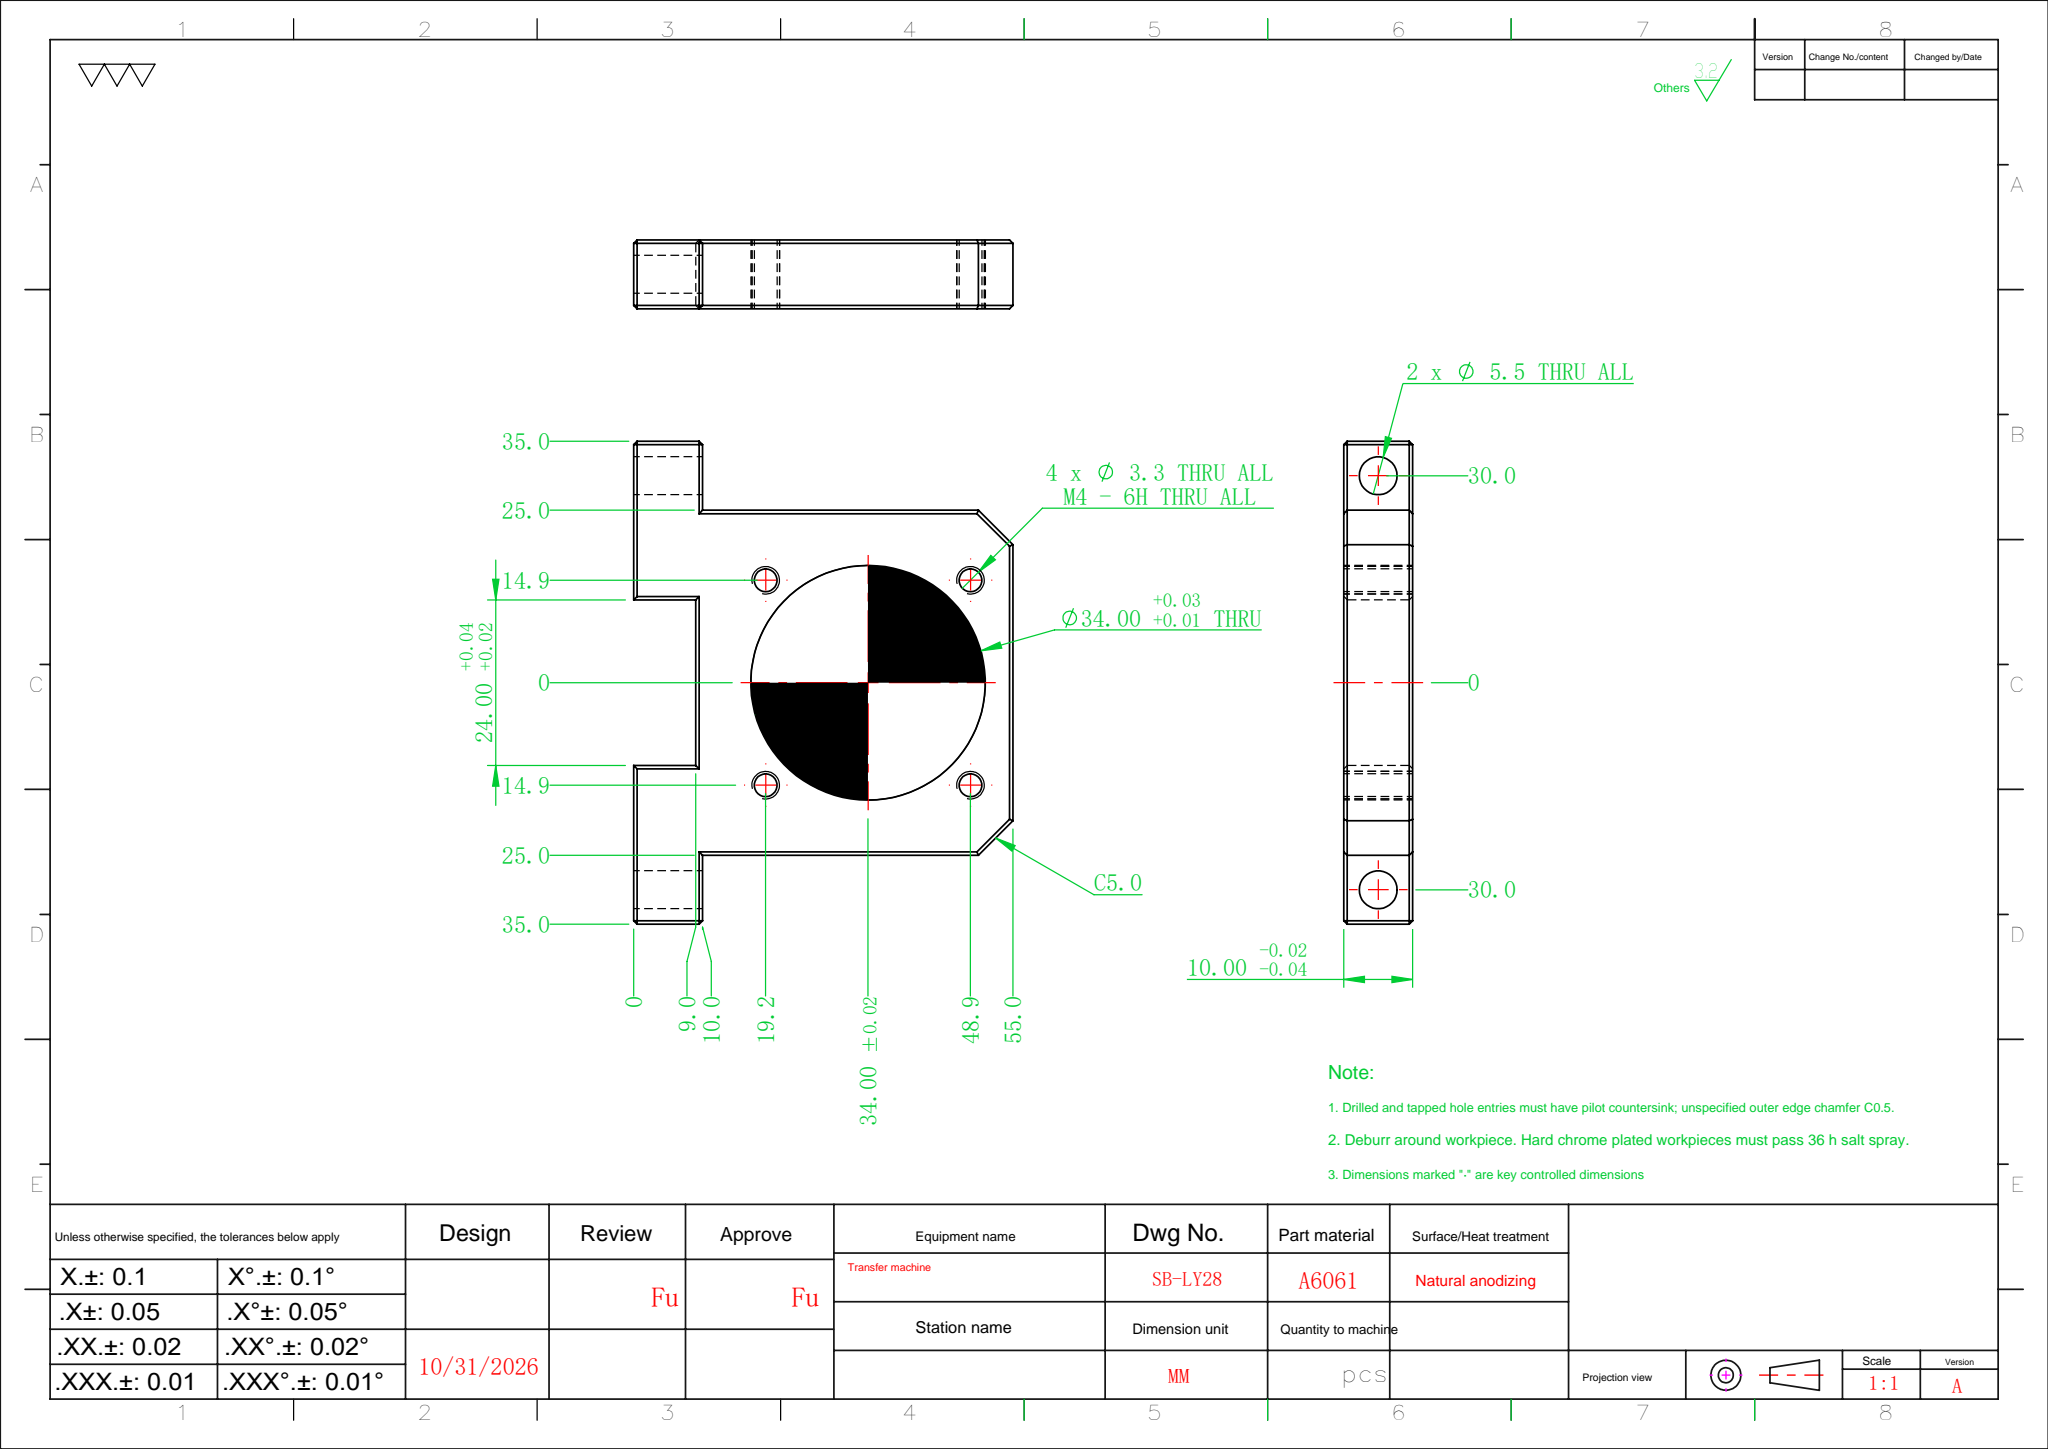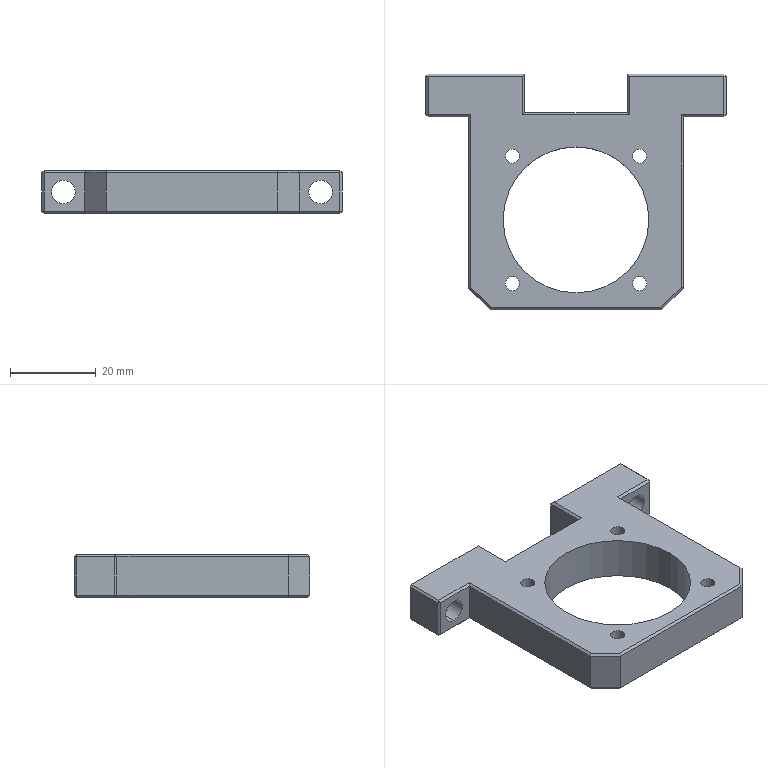Part | SolidWorks | features Chamfer 2, Cut 2, HoleWzd 2, Extrusion 1, ICE 1 | 1 solid | 70 faces | box 70 x 55 x 10 mm | volume 17124 mm3 | plane 56 | cylinder 14 | commonest cylinder face diameters 3.3 x8 5.5 x4 34 x2